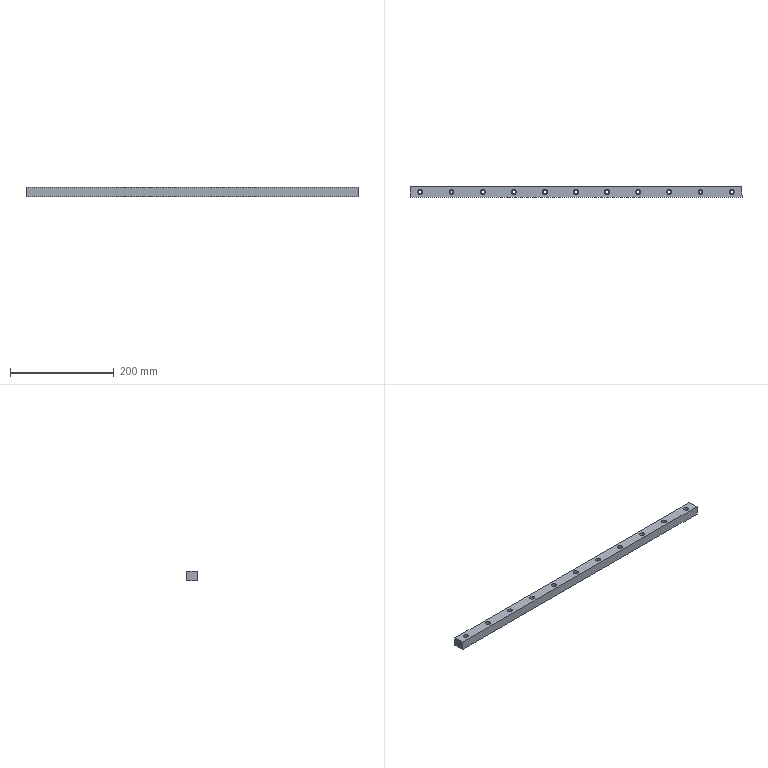Part | STEP file | Slide rod | 1 solid | 61 faces | box 640 x 20 x 17.5 mm | volume 214573 mm3 | cylinder 44 | plane 17 | commonest cylinder face diameters 6 x22 9.5 x22